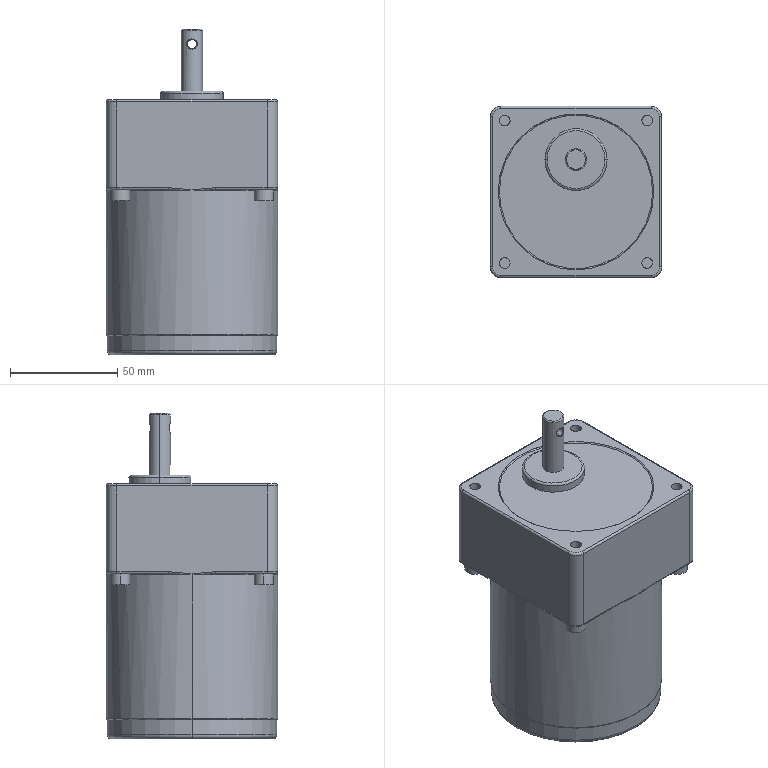Part | STEP file | 102000010051 | 1 solid | 163 faces | box 80 x 80 x 152 mm | volume 650749 mm3 | plane 51 | cylinder 46 | spline 40 | torus 24 | cone 2 | commonest cylinder face diameters 2 x12 5 x8 9 x8 10 x6 4.1 x2 29 x2